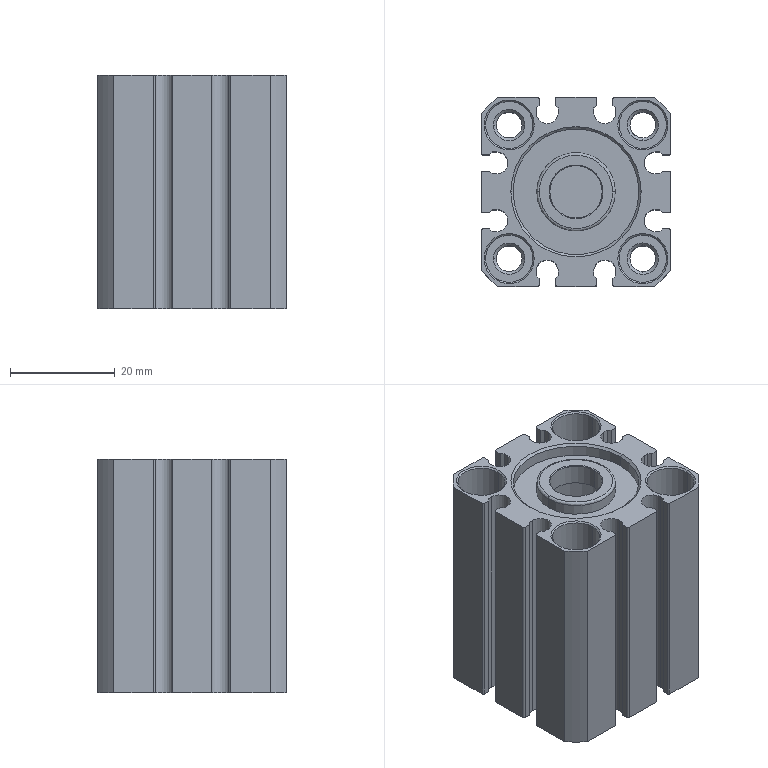Part | STEP file | HI_JSNR20X15_body_default | 1 solid | 198 faces | box 36 x 36 x 44.5 mm | volume 31416 mm3 | plane 78 | cylinder 74 | cone 42 | spline 4 | commonest cylinder face diameters 0.6 x16 9 x16 4.2 x10 4.917 x8 1.5 x4 4.134 x4